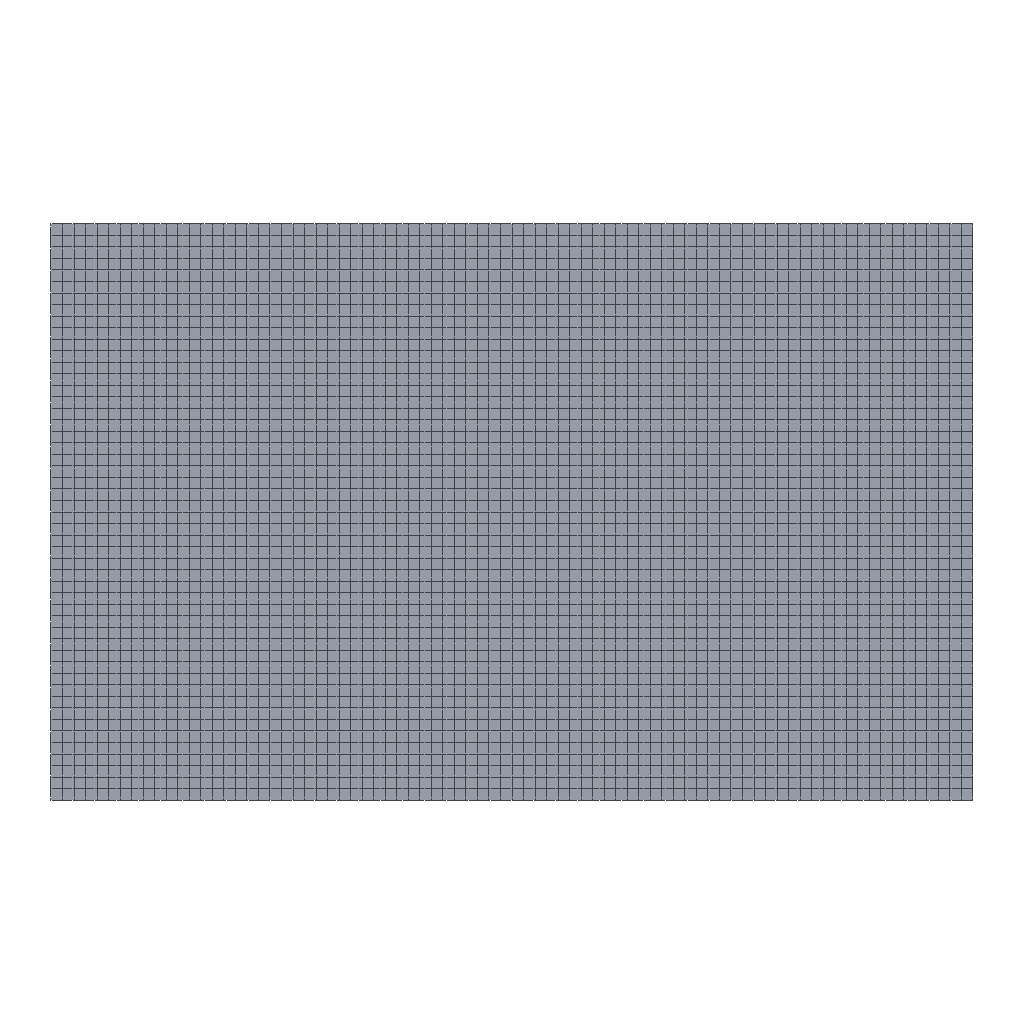Simulation study | abaqus
Set-up summary:
category,name,step,type,value,unit,region
solver,abaqus
solver,version,,,Abaqus/Standard 2020
units,not stated in the deck,,not stated
analysis,deck,,geostatic,geostatic
load_step,Step-1,Step-1,geostatic
load_step,Step-2,Step-2,soils
load_step,requested,,,2
mesh,nodes,,,4164
mesh,elements,,,4030
element_type,T2D2,,truss,30
element_type,CPE4P,,plane,4000
load,load commands in deck,,count,2
bc,support commands in deck,,count,5
material,CRACK,,in results
material,ROCK,,in results
check,setup vs results,,match,"per instance, exact: element labels, types and connectivity; labels of the nodes the elements use; coordinates of those nodes at SINGLE_PRECISION in 2 of 2 instance(s)"
Abaqus input file, long lists of numbers shortened:
*Heading
** Job name: Job-1 Model name: Model-1
** Generated by: Abaqus/CAE 2020
*Preprint, echo=NO, model=NO, history=NO, contact=NO
**
** PARTS
**
*Part, name=CRACK
*Node
      1,         -25.,          -4.
      2,         -25.,          -5.
** (31 more lines like these left out)
*Element, type=T2D2
 1,  1,  7
 2,  7,  8
** (28 more lines like these left out)
*Nset, nset=Set-1, generate
  1,  33,   1
*Elset, elset=Set-1, generate
  1,  30,   1
*Nset, nset=Set-4, generate
  1,  33,   1
*Elset, elset=Set-4, generate
  1,  30,   1
*Nset, nset=Set-5, generate
  1,  33,   1
*Elset, elset=Set-5, generate
  1,  30,   1
** Section: crack
*Solid Section, elset=Set-4, material=CRACK
1.,
*End Part
**
*Part, name=ROCK
*Node
      1,        58.75,        31.25
      2,        57.75,        31.25
** (4129 more lines like these left out)
*Element, type=CPE4P
   1,    1,    2,   83,   82
   2,    2,    3,   84,   83
** (3998 more lines like these left out)
*Nset, nset=Set-1, generate
    1,  4131,     1
*Elset, elset=Set-1, generate
    1,  4000,     1
** Section: rock
*Solid Section, elset=Set-1, material=rock
,
*End Part
**
**
** ASSEMBLY
**
*Assembly, name=Assembly
**
*Instance, name=CRACK-1, part=CRACK
       43.25,       -13.75,           0.
*End Instance
**
*Instance, name=ROCK-1, part=ROCK
*End Instance
**
*Nset, nset=Set-3, instance=CRACK-1, generate
  1,  33,   1
*Nset, nset=Set-3, instance=ROCK-1
    1,   81,   82,  162,  163,  243,  244,  324,  325,  405,  406,  486,  487,  567,  568,  648
  649,  729,  730,  810,  811,  891,  892,  972,  973, 1053, 1054, 1134, 1135, 1215, 1216, 1296
** (5 more lines like these left out)
*Elset, elset=Set-3, instance=CRACK-1, generate
  1,  30,   1
*Elset, elset=Set-3, instance=ROCK-1
    1,   80,   81,  160,  161,  240,  241,  320,  321,  400,  401,  480,  481,  560,  561,  640
  641,  720,  721,  800,  801,  880,  881,  960,  961, 1040, 1041, 1120, 1121, 1200, 1201, 1280
** (5 more lines like these left out)
*Nset, nset=Set-4, instance=CRACK-1, generate
  1,  33,   1
*Nset, nset=Set-4, instance=ROCK-1
    1,   81,   82,  162,  163,  243,  244,  324,  325,  405,  406,  486,  487,  567,  568,  648
  649,  729,  730,  810,  811,  891,  892,  972,  973, 1053, 1054, 1134, 1135, 1215, 1216, 1296
** (5 more lines like these left out)
*Elset, elset=Set-4, instance=CRACK-1, generate
  1,  30,   1
*Elset, elset=Set-4, instance=ROCK-1
    1,   80,   81,  160,  161,  240,  241,  320,  321,  400,  401,  480,  481,  560,  561,  640
  641,  720,  721,  800,  801,  880,  881,  960,  961, 1040, 1041, 1120, 1121, 1200, 1201, 1280
** (5 more lines like these left out)
*Nset, nset=Set-5, instance=ROCK-1
    1,   81,   82,  162,  163,  243,  244,  324,  325,  405,  406,  486,  487,  567,  568,  648
  649,  729,  730,  810,  811,  891,  892,  972,  973, 1053, 1054, 1134, 1135, 1215, 1216, 1296
** (5 more lines like these left out)
*Elset, elset=Set-5, instance=ROCK-1
    1,   80,   81,  160,  161,  240,  241,  320,  321,  400,  401,  480,  481,  560,  561,  640
  641,  720,  721,  800,  801,  880,  881,  960,  961, 1040, 1041, 1120, 1121, 1200, 1201, 1280
** (5 more lines like these left out)
*Nset, nset=Set-7, instance=CRACK-1, generate
  1,  33,   1
*Nset, nset=Set-7, instance=ROCK-1
    1,   81,   82,  162,  163,  243,  244,  324,  325,  405,  406,  486,  487,  567,  568,  648
  649,  729,  730,  810,  811,  891,  892,  972,  973, 1053, 1054, 1134, 1135, 1215, 1216, 1296
** (5 more lines like these left out)
*Elset, elset=Set-7, instance=CRACK-1, generate
  1,  30,   1
*Elset, elset=Set-7, instance=ROCK-1
    1,   80,   81,  160,  161,  240,  241,  320,  321,  400,  401,  480,  481,  560,  561,  640
  641,  720,  721,  800,  801,  880,  881,  960,  961, 1040, 1041, 1120, 1121, 1200, 1201, 1280
** (5 more lines like these left out)
*Nset, nset=Set-8, instance=ROCK-1
    1,   81,   82,  162,  163,  243,  244,  324,  325,  405,  406,  486,  487,  567,  568,  648
  649,  729,  730,  810,  811,  891,  892,  972,  973, 1053, 1054, 1134, 1135, 1215, 1216, 1296
** (5 more lines like these left out)
*Elset, elset=Set-8, instance=ROCK-1
    1,   80,   81,  160,  161,  240,  241,  320,  321,  400,  401,  480,  481,  560,  561,  640
  641,  720,  721,  800,  801,  880,  881,  960,  961, 1040, 1041, 1120, 1121, 1200, 1201, 1280
** (5 more lines like these left out)
*Nset, nset=Set-9, instance=ROCK-1, generate
    1,  4131,     1
*Elset, elset=Set-9, instance=ROCK-1, generate
    1,  4000,     1
*Nset, nset=Set-10, instance=ROCK-1
    1,    2,    3,    4,    5,    6,    7,    8,    9,   10,   11,   12,   13,   14,   15,   16
   17,   18,   19,   20,   21,   22,   23,   24,   25,   26,   27,   28,   29,   30,   31,   32
** (9 more lines like these left out)
*Elset, elset=Set-10, instance=ROCK-1
    1,    2,    3,    4,    5,    6,    7,    8,    9,   10,   11,   12,   13,   14,   15,   16
   17,   18,   19,   20,   21,   22,   23,   24,   25,   26,   27,   28,   29,   30,   31,   32
** (8 more lines like these left out)
*Nset, nset=Set-11, instance=CRACK-1, generate
  1,  33,   1
*Nset, nset=Set-11, instance=ROCK-1, generate
    1,  4131,     1
*Elset, elset=Set-11, instance=CRACK-1, generate
  1,  30,   1
*Elset, elset=Set-11, instance=ROCK-1, generate
    1,  4000,     1
*Nset, nset=Set-12, instance=CRACK-1, generate
  1,  33,   1
*Nset, nset=Set-12, instance=ROCK-1, generate
    1,  4131,     1
*Elset, elset=Set-12, instance=CRACK-1, generate
  1,  30,   1
*Elset, elset=Set-12, instance=ROCK-1, generate
    1,  4000,     1
*Nset, nset=Set-13, instance=ROCK-1
    1,    2,    3,    4,    5,    6,    7,    8,    9,   10,   11,   12,   13,   14,   15,   16
   17,   18,   19,   20,   21,   22,   23,   24,   25,   26,   27,   28,   29,   30,   31,   32
** (9 more lines like these left out)
*Elset, elset=Set-13, instance=ROCK-1
    1,    2,    3,    4,    5,    6,    7,    8,    9,   10,   11,   12,   13,   14,   15,   16
   17,   18,   19,   20,   21,   22,   23,   24,   25,   26,   27,   28,   29,   30,   31,   32
** (8 more lines like these left out)
*Nset, nset=Set-14, instance=ROCK-1
    1,    2,    3,    4,    5,    6,    7,    8,    9,   10,   11,   12,   13,   14,   15,   16
   17,   18,   19,   20,   21,   22,   23,   24,   25,   26,   27,   28,   29,   30,   31,   32
** (9 more lines like these left out)
*Elset, elset=Set-14, instance=ROCK-1
    1,    2,    3,    4,    5,    6,    7,    8,    9,   10,   11,   12,   13,   14,   15,   16
   17,   18,   19,   20,   21,   22,   23,   24,   25,   26,   27,   28,   29,   30,   31,   32
** (8 more lines like these left out)
*Nset, nset=_PickedSet7, internal, instance=CRACK-1, generate
  1,  33,   1
*Elset, elset=_PickedSet7, internal, instance=CRACK-1, generate
  1,  30,   1
*Nset, nset=_PickedSet16, internal, instance=ROCK-1, generate
    1,  4131,     1
*Elset, elset=_PickedSet16, internal, instance=ROCK-1, generate
    1,  4000,     1
*Elset, elset=_Surf-1_S3, internal, instance=ROCK-1, generate
 3921,  4000,     1
*Surface, type=ELEMENT, name=Surf-1
_Surf-1_S3, S3
*Elset, elset=_Surf-2_S3, internal, instance=ROCK-1, generate
 3921,  4000,     1
*Surface, type=ELEMENT, name=Surf-2
_Surf-2_S3, S3
*Nset, nset=Set-8_PP_, internal, instance=ROCK-1
    1,   81,   82,  162,  163,  243,  244,  324,  325,  405,  406,  486,  487,  567,  568,  648
  649,  729,  730,  810,  811,  891,  892,  972,  973, 1053, 1054, 1134, 1135, 1215, 1216, 1296
** (5 more lines like these left out)
*Enrichment, name=Crack-1, type=PROPAGATION CRACK, elset=_PickedSet16
*End Assembly
*Amplitude, name=Amp-1
             0.,              0.,              1.,             0.5,              2.,              1.
**
** MATERIALS
**
*Material, name=CRACK
*Elastic
 1e+10, 0.28
*Material, name=rock
*Damage Initiation, criterion=MAXPS
 4e+06,
*Damage Evolution, type=ENERGY, mixed mode behavior=POWER LAW, power=2.
8000.,8000.,8000.
*Damage Stabilization
0.0001
*Elastic
 1.5e+10, 0.25
*Fluid Leakoff
 5e-14, 1e-14
*Gap Flow
 0.0001,
*Permeability, specific=9800.
 1e-07, 0.1
*Initial Conditions, type=ENRICHMENT
ROCK-1.395, 1,Crack-1, 0.5, 0.
ROCK-1.395, 2,Crack-1, -0.5, 0.
ROCK-1.395, 3,Crack-1, -0.5, -1.
ROCK-1.395, 4,Crack-1, 0.5, -1.
ROCK-1.396, 1,Crack-1, 0.5, 0.
ROCK-1.396, 2,Crack-1, -0.5, 0.
ROCK-1.396, 3,Crack-1, -0.5, -1.
ROCK-1.396, 4,Crack-1, 0.5, -1.
ROCK-1.397, 1,Crack-1, 0.5, 0.
ROCK-1.397, 2,Crack-1, -0.5, 0.
ROCK-1.397, 3,Crack-1, -0.5, -1.
ROCK-1.397, 4,Crack-1, 0.5, -1.
**
** BOUNDARY CONDITIONS
**
** Name: BC-1 Type: 位移/转角
*Boundary
Set-5, 1, 1
** Name: BC-3 Type: 孔隙压力
*Boundary
Set-8_PP_, 8, 8
** Name: BC-5 Type: 位移/转角
*Boundary
Set-14, 2, 2
**
** PREDEFINED FIELDS
**
** Name: Predefined Field-1   Type: Void ratio
*Initial Conditions, TYPE=RATIO
Set-11, 0.1
** Name: Predefined Field-2   Type: Pore pressure
*Initial Conditions, TYPE=PORE PRESSURE
Set-12, 2e+07
** Name: Predefined Field-3   Type: Stress
*Initial Conditions, type=STRESS
Set-9, -2.4e+07, -2.1e+07, -2.1e+07, 0.,
** ----------------------------------------------------------------
**
** STEP: Step-1
**
*Step, name=Step-1, nlgeom=YES, unsymm=YES
*Geostatic
**
** BOUNDARY CONDITIONS
**
** Name: BC-4 Type: 位移/转角
*Boundary
Set-13, 2, 2
**
** OUTPUT REQUESTS
**
*Restart, write, frequency=0
**
** FIELD OUTPUT: F-Output-1
**
*Output, field
*Node Output
CF, PHILSM, POR, PSILSM, RF, U, V
*Element Output, directions=YES
FLVEL, LE, MISES, S, SAT, VOIDR
*Contact Output
CDISP, CSTRESS
**
** HISTORY OUTPUT: H-Output-1
**
*Output, history, variable=PRESELECT
*End Step
** ----------------------------------------------------------------
**
** STEP: Step-2
**
*Step, name=Step-2, nlgeom=YES, inc=100000, unsymm=YES
*Soils, consolidation, end=PERIOD, utol=1e+09, stabilize=0.0002, allsdtol=0.05, continue=NO
0.1, 10., 1e-07, 1.,
**
** BOUNDARY CONDITIONS
**
** Name: BC-3 Type: 孔隙压力
*Boundary
Set-8_PP_, 8, 8, 1e+07
**
** LOADS
**
** Name: Load-1   Type: Pressure
*Dsload
Surf-2, P, 2e+07
**
** CONTROLS
**
*Controls, reset
*Controls, parameters=time incrementation
, , , , , , , 20, , ,
**
** OUTPUT REQUESTS
**
*Restart, write, frequency=0
**
** FIELD OUTPUT: F-Output-1, F-Output-2
**
*Output, field
*Node Output
CF, PHILSM, POR, PSILSM, RF, U, V
*Element Output, directions=YES
FLVEL, LE, MISES, S, SAT, VOIDR
*Contact Output
CDISP, CSTRESS
**
** HISTORY OUTPUT: H-Output-1
**
*Output, history, variable=PRESELECT
*End Step
Results summary:
result,step,,completed,increments=1 time=1.0/1.0
result,step,,completed,increments=20 time=10.0/10.0
result,analysis,,,"soils, consolidation"
result,last_loadstep,,,2
result,primary field,,,"U, POR"
result,reaction total,,FX,-14.0,model units
result,reaction total,,FY,-1599999994.0,model units
result,reaction total,,FZ,0.0,model units